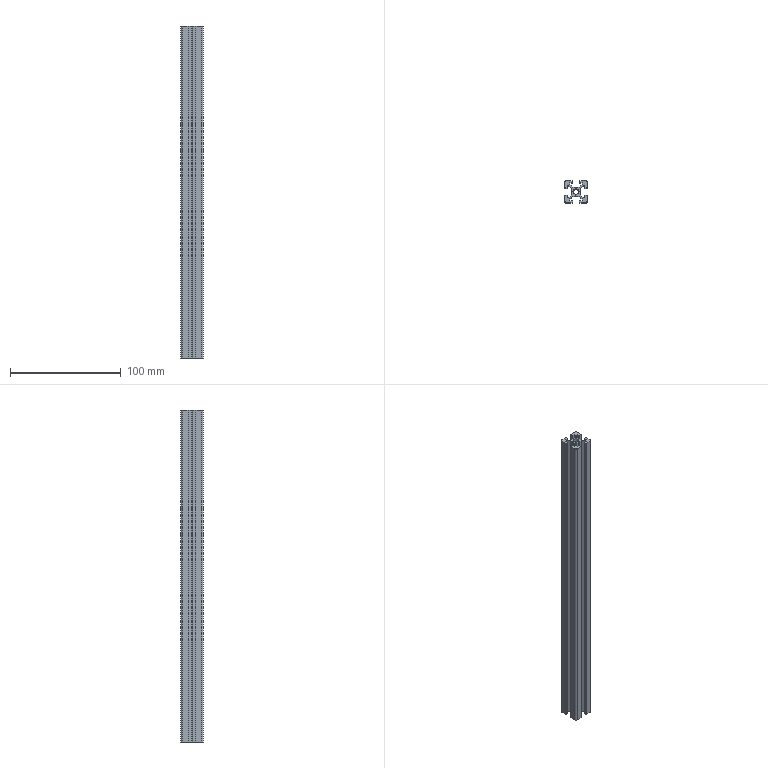Part | STEP file | AOB02-H2020_YHD016 | 1 solid | 80 faces | box 20 x 20 x 300 mm | volume 51792 mm3 | plane 74 | cylinder 6 | commonest cylinder face diameters 3 x4 5 x2